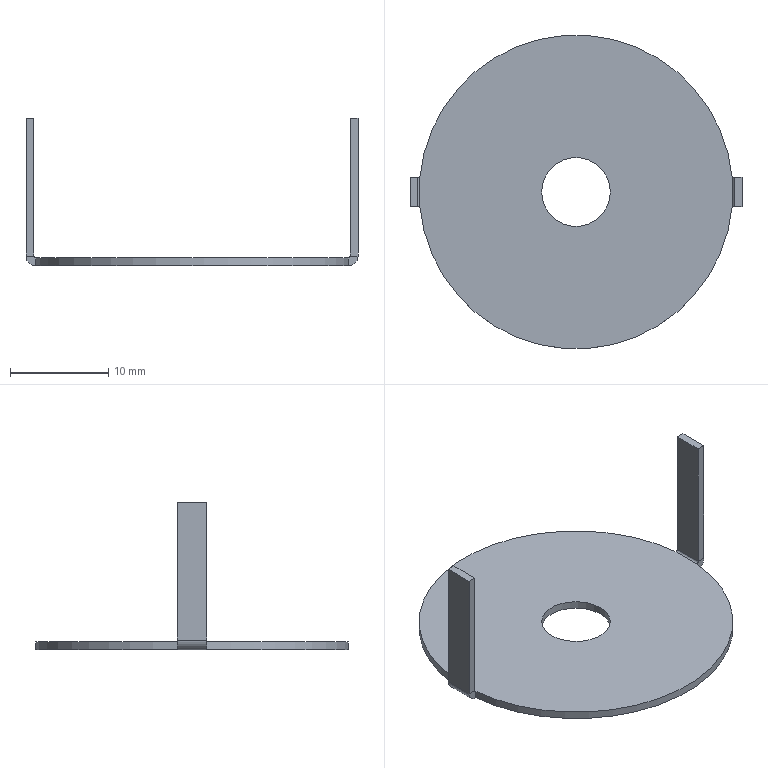Part | STEP file | Q7C1215W | 1 solid | 23 faces | box 33.859 x 32 x 15.058 mm | volume 684.385 mm3 | plane 16 | cylinder 7 | commonest cylinder face diameters 0.4 x2 2 x2 32 x2 7 x1
STEP:
#1=CARTESIAN_POINT('',(0.,0.,0.));
#2=DIRECTION('',(0.,0.,1.));
#3=DIRECTION('',(1.,0.,0.));
#4=AXIS2_PLACEMENT_3D('',#1,#2,#3);
#5=CARTESIAN_POINT('',(3.5,0.,0.));
#6=VERTEX_POINT('',#5);
#7=CARTESIAN_POINT('',(0.,0.,0.));
#8=DIRECTION('',(0.,0.,1.));
#9=DIRECTION('',(1.,0.,0.));
#10=AXIS2_PLACEMENT_3D('',#7,#8,#9);
#11=CIRCLE('',#10,3.5);
#12=CARTESIAN_POINT('',(0.,0.,0.));
#13=DIRECTION('',(0.,0.,1.));
#14=DIRECTION('',(1.,0.,0.));
#15=AXIS2_PLACEMENT_3D('',#12,#13,#14);
#16=PLANE('',#15);
#17=CARTESIAN_POINT('',(0.,0.));
#18=DIRECTION('',(1.,0.));
#19=AXIS2_PLACEMENT_2D('',#17,#18);
#20=CIRCLE('',#19,3.5);
#21=(GEOMETRIC_REPRESENTATION_CONTEXT(2)PARAMETRIC_REPRESENTATION_CONTEXT()REPRESENTATION_CONTEXT('',''));
#22=DEFINITIONAL_REPRESENTATION('',(#20),#21);
#23=PCURVE('',#16,#22);
#24=CARTESIAN_POINT('',(0.,0.,-0.8));
#25=DIRECTION('',(0.,0.,1.));
#26=DIRECTION('',(1.,0.,0.));
#27=AXIS2_PLACEMENT_3D('',#24,#25,#26);
#28=CYLINDRICAL_SURFACE('',#27,3.5);
#29=CARTESIAN_POINT('',(0.,0.8));
#30=DIRECTION('',(1.,0.));
#31=VECTOR('',#30,1.);
#32=LINE('',#29,#31);
#33=(GEOMETRIC_REPRESENTATION_CONTEXT(2)PARAMETRIC_REPRESENTATION_CONTEXT()REPRESENTATION_CONTEXT('',''));
#34=DEFINITIONAL_REPRESENTATION('',(#32),#33);
#35=PCURVE('',#28,#34);
#36=SURFACE_CURVE('',#11,(#23,#35),.PCURVE_S1.);
#37=EDGE_CURVE('',#6,#6,#36,.T.);
#38=ORIENTED_EDGE('',*,*,#37,.F.);
#39=EDGE_LOOP('',(#38));
#40=FACE_BOUND('',#39,.T.);
#41=CARTESIAN_POINT('',(-15.93,-1.5,0.));
#42=VERTEX_POINT('',#41);
#43=CARTESIAN_POINT('',(15.93,-1.5,0.));
#44=VERTEX_POINT('',#43);
#45=CARTESIAN_POINT('',(0.,0.,0.));
#46=DIRECTION('',(0.,0.,1.));
#47=DIRECTION('',(1.,0.,0.));
#48=AXIS2_PLACEMENT_3D('',#45,#46,#47);
#49=CIRCLE('',#48,16.);
#50=CARTESIAN_POINT('',(0.,0.));
#51=DIRECTION('',(1.,0.));
#52=AXIS2_PLACEMENT_2D('',#50,#51);
#53=CIRCLE('',#52,16.);
#54=(GEOMETRIC_REPRESENTATION_CONTEXT(2)PARAMETRIC_REPRESENTATION_CONTEXT()REPRESENTATION_CONTEXT('',''));
#55=DEFINITIONAL_REPRESENTATION('',(#53),#54);
#56=PCURVE('',#16,#55);
#57=CARTESIAN_POINT('',(0.,0.,-0.8));
#58=DIRECTION('',(0.,0.,1.));
#59=DIRECTION('',(1.,0.,0.));
#60=AXIS2_PLACEMENT_3D('',#57,#58,#59);
#61=CYLINDRICAL_SURFACE('',#60,16.);
#62=CARTESIAN_POINT('',(0.,0.8));
#63=DIRECTION('',(1.,0.));
#64=VECTOR('',#63,1.);
#65=LINE('',#62,#64);
#66=(GEOMETRIC_REPRESENTATION_CONTEXT(2)PARAMETRIC_REPRESENTATION_CONTEXT()REPRESENTATION_CONTEXT('',''));
#67=DEFINITIONAL_REPRESENTATION('',(#65),#66);
#68=PCURVE('',#61,#67);
#69=SURFACE_CURVE('',#49,(#56,#68),.PCURVE_S1.);
#70=EDGE_CURVE('',#42,#44,#69,.T.);
#71=ORIENTED_EDGE('',*,*,#70,.T.);
#72=CARTESIAN_POINT('',(15.93,1.5,0.));
#73=VERTEX_POINT('',#72);
#74=CARTESIAN_POINT('',(15.93,0.,0.));
#75=DIRECTION('',(0.,1.,0.));
#76=VECTOR('',#75,1.);
#77=LINE('',#74,#76);
#78=CARTESIAN_POINT('',(15.93,0.));
#79=DIRECTION('',(0.,1.));
#80=VECTOR('',#79,1.);
#81=LINE('',#78,#80);
#82=(GEOMETRIC_REPRESENTATION_CONTEXT(2)PARAMETRIC_REPRESENTATION_CONTEXT()REPRESENTATION_CONTEXT('',''));
#83=DEFINITIONAL_REPRESENTATION('',(#81),#82);
#84=PCURVE('',#16,#83);
#85=CARTESIAN_POINT('',(15.93,3.245,0.2));
#86=DIRECTION('',(0.,-1.,0.));
#87=DIRECTION('',(0.,0.,-1.));
#88=AXIS2_PLACEMENT_3D('',#85,#86,#87);
#89=CYLINDRICAL_SURFACE('',#88,0.2);
#90=CARTESIAN_POINT('',(0.,3.245));
#91=DIRECTION('',(0.,-1.));
#92=VECTOR('',#91,1.);
#93=LINE('',#90,#92);
#94=(GEOMETRIC_REPRESENTATION_CONTEXT(2)PARAMETRIC_REPRESENTATION_CONTEXT()REPRESENTATION_CONTEXT('',''));
#95=DEFINITIONAL_REPRESENTATION('',(#93),#94);
#96=PCURVE('',#89,#95);
#97=SURFACE_CURVE('',#77,(#84,#96),.PCURVE_S1.);
#98=EDGE_CURVE('',#44,#73,#97,.T.);
#99=ORIENTED_EDGE('',*,*,#98,.T.);
#100=CARTESIAN_POINT('',(-15.93,1.5,0.));
#101=VERTEX_POINT('',#100);
#102=CARTESIAN_POINT('',(0.,0.,0.));
#103=DIRECTION('',(0.,0.,1.));
#104=DIRECTION('',(1.,0.,0.));
#105=AXIS2_PLACEMENT_3D('',#102,#103,#104);
#106=CIRCLE('',#105,16.);
#107=CARTESIAN_POINT('',(0.,0.));
#108=DIRECTION('',(1.,0.));
#109=AXIS2_PLACEMENT_2D('',#107,#108);
#110=CIRCLE('',#109,16.);
#111=(GEOMETRIC_REPRESENTATION_CONTEXT(2)PARAMETRIC_REPRESENTATION_CONTEXT()REPRESENTATION_CONTEXT('',''));
#112=DEFINITIONAL_REPRESENTATION('',(#110),#111);
#113=PCURVE('',#16,#112);
#114=CARTESIAN_POINT('',(0.,0.,-0.8));
#115=DIRECTION('',(0.,0.,1.));
#116=DIRECTION('',(1.,0.,0.));
#117=AXIS2_PLACEMENT_3D('',#114,#115,#116);
#118=CYLINDRICAL_SURFACE('',#117,16.);
#119=CARTESIAN_POINT('',(0.,0.8));
#120=DIRECTION('',(1.,0.));
#121=VECTOR('',#120,1.);
#122=LINE('',#119,#121);
#123=(GEOMETRIC_REPRESENTATION_CONTEXT(2)PARAMETRIC_REPRESENTATION_CONTEXT()REPRESENTATION_CONTEXT('',''));
#124=DEFINITIONAL_REPRESENTATION('',(#122),#123);
#125=PCURVE('',#118,#124);
#126=SURFACE_CURVE('',#106,(#113,#125),.PCURVE_S1.);
#127=EDGE_CURVE('',#73,#101,#126,.T.);
#128=ORIENTED_EDGE('',*,*,#127,.T.);
#129=CARTESIAN_POINT('',(-15.93,0.,0.));
#130=DIRECTION('',(0.,1.,0.));
#131=VECTOR('',#130,1.);
#132=LINE('',#129,#131);
#133=CARTESIAN_POINT('',(-15.93,0.));
#134=DIRECTION('',(0.,1.));
#135=VECTOR('',#134,1.);
#136=LINE('',#133,#135);
#137=(GEOMETRIC_REPRESENTATION_CONTEXT(2)PARAMETRIC_REPRESENTATION_CONTEXT()REPRESENTATION_CONTEXT('',''));
#138=DEFINITIONAL_REPRESENTATION('',(#136),#137);
#139=PCURVE('',#16,#138);
#140=CARTESIAN_POINT('',(-15.93,-3.245,0.2));
#141=DIRECTION('',(0.,1.,0.));
#142=DIRECTION('',(0.,0.,1.));
#143=AXIS2_PLACEMENT_3D('',#140,#141,#142);
#144=CYLINDRICAL_SURFACE('',#143,0.2);
#145=CARTESIAN_POINT('',(3.142,3.245));
#146=DIRECTION('',(0.,1.));
#147=VECTOR('',#146,1.);
#148=LINE('',#145,#147);
#149=(GEOMETRIC_REPRESENTATION_CONTEXT(2)PARAMETRIC_REPRESENTATION_CONTEXT()REPRESENTATION_CONTEXT('',''));
#150=DEFINITIONAL_REPRESENTATION('',(#148),#149);
#151=PCURVE('',#144,#150);
#152=SURFACE_CURVE('',#132,(#139,#151),.PCURVE_S1.);
#153=EDGE_CURVE('',#42,#101,#152,.T.);
#154=ORIENTED_EDGE('',*,*,#153,.F.);
#155=EDGE_LOOP('',(#71,#99,#128,#154));
#156=FACE_BOUND('',#155,.T.);
#157=ADVANCED_FACE('',(#40,#156),#16,.T.);
#158=CARTESIAN_POINT('',(15.93,-1.5,-0.8));
#159=VERTEX_POINT('',#158);
#160=CARTESIAN_POINT('',(15.93,1.5,-0.8));
#161=VERTEX_POINT('',#160);
#162=CARTESIAN_POINT('',(15.93,0.,-0.8));
#163=DIRECTION('',(0.,1.,0.));
#164=VECTOR('',#163,1.);
#165=LINE('',#162,#164);
#166=CARTESIAN_POINT('',(0.,0.,-0.8));
#167=DIRECTION('',(0.,0.,1.));
#168=DIRECTION('',(1.,0.,0.));
#169=AXIS2_PLACEMENT_3D('',#166,#167,#168);
#170=PLANE('',#169);
#171=CARTESIAN_POINT('',(15.93,0.));
#172=DIRECTION('',(0.,1.));
#173=VECTOR('',#172,1.);
#174=LINE('',#171,#173);
#175=(GEOMETRIC_REPRESENTATION_CONTEXT(2)PARAMETRIC_REPRESENTATION_CONTEXT()REPRESENTATION_CONTEXT('',''));
#176=DEFINITIONAL_REPRESENTATION('',(#174),#175);
#177=PCURVE('',#170,#176);
#178=CARTESIAN_POINT('',(15.93,3.245,0.2));
#179=DIRECTION('',(0.,-1.,0.));
#180=DIRECTION('',(0.,0.,-1.));
#181=AXIS2_PLACEMENT_3D('',#178,#179,#180);
#182=CYLINDRICAL_SURFACE('',#181,1.);
#183=CARTESIAN_POINT('',(0.,3.245));
#184=DIRECTION('',(0.,-1.));
#185=VECTOR('',#184,1.);
#186=LINE('',#183,#185);
#187=(GEOMETRIC_REPRESENTATION_CONTEXT(2)PARAMETRIC_REPRESENTATION_CONTEXT()REPRESENTATION_CONTEXT('',''));
#188=DEFINITIONAL_REPRESENTATION('',(#186),#187);
#189=PCURVE('',#182,#188);
#190=SURFACE_CURVE('',#165,(#177,#189),.PCURVE_S1.);
#191=EDGE_CURVE('',#159,#161,#190,.T.);
#192=ORIENTED_EDGE('',*,*,#191,.F.);
#193=CARTESIAN_POINT('',(-15.93,-1.5,-0.8));
#194=VERTEX_POINT('',#193);
#195=CARTESIAN_POINT('',(0.,0.,-0.8));
#196=DIRECTION('',(0.,0.,1.));
#197=DIRECTION('',(1.,0.,0.));
#198=AXIS2_PLACEMENT_3D('',#195,#196,#197);
#199=CIRCLE('',#198,16.);
#200=CARTESIAN_POINT('',(0.,0.));
#201=DIRECTION('',(1.,0.));
#202=AXIS2_PLACEMENT_2D('',#200,#201);
#203=CIRCLE('',#202,16.);
#204=(GEOMETRIC_REPRESENTATION_CONTEXT(2)PARAMETRIC_REPRESENTATION_CONTEXT()REPRESENTATION_CONTEXT('',''));
#205=DEFINITIONAL_REPRESENTATION('',(#203),#204);
#206=PCURVE('',#170,#205);
#207=CARTESIAN_POINT('',(0.,0.));
#208=DIRECTION('',(1.,0.));
#209=VECTOR('',#208,1.);
#210=LINE('',#207,#209);
#211=(GEOMETRIC_REPRESENTATION_CONTEXT(2)PARAMETRIC_REPRESENTATION_CONTEXT()REPRESENTATION_CONTEXT('',''));
#212=DEFINITIONAL_REPRESENTATION('',(#210),#211);
#213=PCURVE('',#61,#212);
#214=SURFACE_CURVE('',#199,(#206,#213),.PCURVE_S1.);
#215=EDGE_CURVE('',#194,#159,#214,.T.);
#216=ORIENTED_EDGE('',*,*,#215,.F.);
#217=CARTESIAN_POINT('',(-15.93,1.5,-0.8));
#218=VERTEX_POINT('',#217);
#219=CARTESIAN_POINT('',(-15.93,0.,-0.8));
#220=DIRECTION('',(0.,1.,0.));
#221=VECTOR('',#220,1.);
#222=LINE('',#219,#221);
#223=CARTESIAN_POINT('',(-15.93,0.));
#224=DIRECTION('',(0.,1.));
#225=VECTOR('',#224,1.);
#226=LINE('',#223,#225);
#227=(GEOMETRIC_REPRESENTATION_CONTEXT(2)PARAMETRIC_REPRESENTATION_CONTEXT()REPRESENTATION_CONTEXT('',''));
#228=DEFINITIONAL_REPRESENTATION('',(#226),#227);
#229=PCURVE('',#170,#228);
#230=CARTESIAN_POINT('',(-15.93,-3.245,0.2));
#231=DIRECTION('',(0.,1.,0.));
#232=DIRECTION('',(0.,0.,1.));
#233=AXIS2_PLACEMENT_3D('',#230,#231,#232);
#234=CYLINDRICAL_SURFACE('',#233,1.);
#235=CARTESIAN_POINT('',(3.142,3.245));
#236=DIRECTION('',(0.,1.));
#237=VECTOR('',#236,1.);
#238=LINE('',#235,#237);
#239=(GEOMETRIC_REPRESENTATION_CONTEXT(2)PARAMETRIC_REPRESENTATION_CONTEXT()REPRESENTATION_CONTEXT('',''));
#240=DEFINITIONAL_REPRESENTATION('',(#238),#239);
#241=PCURVE('',#234,#240);
#242=SURFACE_CURVE('',#222,(#229,#241),.PCURVE_S1.);
#243=EDGE_CURVE('',#194,#218,#242,.T.);
#244=ORIENTED_EDGE('',*,*,#243,.T.);
#245=CARTESIAN_POINT('',(0.,0.,-0.8));
#246=DIRECTION('',(0.,0.,1.));
#247=DIRECTION('',(1.,0.,0.));
#248=AXIS2_PLACEMENT_3D('',#245,#246,#247);
#249=CIRCLE('',#248,16.);
#250=CARTESIAN_POINT('',(0.,0.));
#251=DIRECTION('',(1.,0.));
#252=AXIS2_PLACEMENT_2D('',#250,#251);
#253=CIRCLE('',#252,16.);
#254=(GEOMETRIC_REPRESENTATION_CONTEXT(2)PARAMETRIC_REPRESENTATION_CONTEXT()REPRESENTATION_CONTEXT('',''));
#255=DEFINITIONAL_REPRESENTATION('',(#253),#254);
#256=PCURVE('',#170,#255);
#257=CARTESIAN_POINT('',(0.,0.));
#258=DIRECTION('',(1.,0.));
#259=VECTOR('',#258,1.);
#260=LINE('',#257,#259);
#261=(GEOMETRIC_REPRESENTATION_CONTEXT(2)PARAMETRIC_REPRESENTATION_CONTEXT()REPRESENTATION_CONTEXT('',''));
#262=DEFINITIONAL_REPRESENTATION('',(#260),#261);
#263=PCURVE('',#118,#262);
#264=SURFACE_CURVE('',#249,(#256,#263),.PCURVE_S1.);
#265=EDGE_CURVE('',#161,#218,#264,.T.);
#266=ORIENTED_EDGE('',*,*,#265,.F.);
#267=EDGE_LOOP('',(#192,#216,#244,#266));
#268=FACE_BOUND('',#267,.T.);
#269=CARTESIAN_POINT('',(3.5,0.,-0.8));
#270=VERTEX_POINT('',#269);
#271=CARTESIAN_POINT('',(0.,0.,-0.8));
#272=DIRECTION('',(0.,0.,1.));
#273=DIRECTION('',(1.,0.,0.));
#274=AXIS2_PLACEMENT_3D('',#271,#272,#273);
#275=CIRCLE('',#274,3.5);
#276=CARTESIAN_POINT('',(0.,0.));
#277=DIRECTION('',(1.,0.));
#278=AXIS2_PLACEMENT_2D('',#276,#277);
#279=CIRCLE('',#278,3.5);
#280=(GEOMETRIC_REPRESENTATION_CONTEXT(2)PARAMETRIC_REPRESENTATION_CONTEXT()REPRESENTATION_CONTEXT('',''));
#281=DEFINITIONAL_REPRESENTATION('',(#279),#280);
#282=PCURVE('',#170,#281);
#283=CARTESIAN_POINT('',(0.,0.));
#284=DIRECTION('',(1.,0.));
#285=VECTOR('',#284,1.);
#286=LINE('',#283,#285);
#287=(GEOMETRIC_REPRESENTATION_CONTEXT(2)PARAMETRIC_REPRESENTATION_CONTEXT()REPRESENTATION_CONTEXT('',''));
#288=DEFINITIONAL_REPRESENTATION('',(#286),#287);
#289=PCURVE('',#28,#288);
#290=SURFACE_CURVE('',#275,(#282,#289),.PCURVE_S1.);
#291=EDGE_CURVE('',#270,#270,#290,.T.);
#292=ORIENTED_EDGE('',*,*,#291,.T.);
#293=EDGE_LOOP('',(#292));
#294=FACE_BOUND('',#293,.T.);
#295=ADVANCED_FACE('',(#268,#294),#170,.F.);
#296=ORIENTED_EDGE('',*,*,#127,.F.);
#297=CARTESIAN_POINT('',(15.93,1.5,-0.8));
#298=DIRECTION('',(0.,0.,1.));
#299=VECTOR('',#298,1.);
#300=LINE('',#297,#299);
#301=CARTESIAN_POINT('',(0.09389,0.));
#302=DIRECTION('',(0.,1.));
#303=VECTOR('',#302,1.);
#304=LINE('',#301,#303);
#305=(GEOMETRIC_REPRESENTATION_CONTEXT(2)PARAMETRIC_REPRESENTATION_CONTEXT()REPRESENTATION_CONTEXT('',''));
#306=DEFINITIONAL_REPRESENTATION('',(#304),#305);
#307=PCURVE('',#118,#306);
#308=CARTESIAN_POINT('',(15.93,1.5,0.2));
#309=DIRECTION('',(0.,1.,0.));
#310=DIRECTION('',(0.,0.,1.));
#311=AXIS2_PLACEMENT_3D('',#308,#309,#310);
#312=PLANE('',#311);
#313=CARTESIAN_POINT('',(-1.,0.));
#314=DIRECTION('',(1.,0.));
#315=VECTOR('',#314,1.);
#316=LINE('',#313,#315);
#317=(GEOMETRIC_REPRESENTATION_CONTEXT(2)PARAMETRIC_REPRESENTATION_CONTEXT()REPRESENTATION_CONTEXT('',''));
#318=DEFINITIONAL_REPRESENTATION('',(#316),#317);
#319=PCURVE('',#312,#318);
#320=SURFACE_CURVE('',#300,(#307,#319),.PCURVE_S1.);
#321=EDGE_CURVE('',#161,#73,#320,.T.);
#322=ORIENTED_EDGE('',*,*,#321,.F.);
#323=ORIENTED_EDGE('',*,*,#265,.T.);
#324=CARTESIAN_POINT('',(-15.93,1.5,-0.8));
#325=DIRECTION('',(0.,0.,1.));
#326=VECTOR('',#325,1.);
#327=LINE('',#324,#326);
#328=CARTESIAN_POINT('',(3.048,0.));
#329=DIRECTION('',(0.,1.));
#330=VECTOR('',#329,1.);
#331=LINE('',#328,#330);
#332=(GEOMETRIC_REPRESENTATION_CONTEXT(2)PARAMETRIC_REPRESENTATION_CONTEXT()REPRESENTATION_CONTEXT('',''));
#333=DEFINITIONAL_REPRESENTATION('',(#331),#332);
#334=PCURVE('',#118,#333);
#335=CARTESIAN_POINT('',(-15.93,1.5,0.2));
#336=DIRECTION('',(0.,1.,0.));
#337=DIRECTION('',(0.,0.,1.));
#338=AXIS2_PLACEMENT_3D('',#335,#336,#337);
#339=PLANE('',#338);
#340=CARTESIAN_POINT('',(-1.,0.));
#341=DIRECTION('',(1.,0.));
#342=VECTOR('',#341,1.);
#343=LINE('',#340,#342);
#344=(GEOMETRIC_REPRESENTATION_CONTEXT(2)PARAMETRIC_REPRESENTATION_CONTEXT()REPRESENTATION_CONTEXT('',''));
#345=DEFINITIONAL_REPRESENTATION('',(#343),#344);
#346=PCURVE('',#339,#345);
#347=SURFACE_CURVE('',#327,(#334,#346),.PCURVE_S1.);
#348=EDGE_CURVE('',#218,#101,#347,.T.);
#349=ORIENTED_EDGE('',*,*,#348,.T.);
#350=EDGE_LOOP('',(#296,#322,#323,#349));
#351=FACE_BOUND('',#350,.T.);
#352=ADVANCED_FACE('',(#351),#118,.T.);
#353=ORIENTED_EDGE('',*,*,#70,.F.);
#354=CARTESIAN_POINT('',(-15.93,-1.5,-0.8));
#355=DIRECTION('',(0.,0.,1.));
#356=VECTOR('',#355,1.);
#357=LINE('',#354,#356);
#358=CARTESIAN_POINT('',(3.235,0.));
#359=DIRECTION('',(0.,1.));
#360=VECTOR('',#359,1.);
#361=LINE('',#358,#360);
#362=(GEOMETRIC_REPRESENTATION_CONTEXT(2)PARAMETRIC_REPRESENTATION_CONTEXT()REPRESENTATION_CONTEXT('',''));
#363=DEFINITIONAL_REPRESENTATION('',(#361),#362);
#364=PCURVE('',#61,#363);
#365=CARTESIAN_POINT('',(-15.93,-1.5,0.2));
#366=DIRECTION('',(0.,-1.,0.));
#367=DIRECTION('',(0.,0.,-1.));
#368=AXIS2_PLACEMENT_3D('',#365,#366,#367);
#369=PLANE('',#368);
#370=CARTESIAN_POINT('',(1.,0.));
#371=DIRECTION('',(-1.,0.));
#372=VECTOR('',#371,1.);
#373=LINE('',#370,#372);
#374=(GEOMETRIC_REPRESENTATION_CONTEXT(2)PARAMETRIC_REPRESENTATION_CONTEXT()REPRESENTATION_CONTEXT('',''));
#375=DEFINITIONAL_REPRESENTATION('',(#373),#374);
#376=PCURVE('',#369,#375);
#377=SURFACE_CURVE('',#357,(#364,#376),.PCURVE_S1.);
#378=EDGE_CURVE('',#194,#42,#377,.T.);
#379=ORIENTED_EDGE('',*,*,#378,.F.);
#380=ORIENTED_EDGE('',*,*,#215,.T.);
#381=CARTESIAN_POINT('',(15.93,-1.5,-0.8));
#382=DIRECTION('',(0.,0.,1.));
#383=VECTOR('',#382,1.);
#384=LINE('',#381,#383);
#385=CARTESIAN_POINT('',(6.189,0.));
#386=DIRECTION('',(0.,1.));
#387=VECTOR('',#386,1.);
#388=LINE('',#385,#387);
#389=(GEOMETRIC_REPRESENTATION_CONTEXT(2)PARAMETRIC_REPRESENTATION_CONTEXT()REPRESENTATION_CONTEXT('',''));
#390=DEFINITIONAL_REPRESENTATION('',(#388),#389);
#391=PCURVE('',#61,#390);
#392=CARTESIAN_POINT('',(15.93,-1.5,0.2));
#393=DIRECTION('',(0.,-1.,0.));
#394=DIRECTION('',(1.,0.,0.));
#395=AXIS2_PLACEMENT_3D('',#392,#393,#394);
#396=PLANE('',#395);
#397=CARTESIAN_POINT('',(0.,-1.));
#398=DIRECTION('',(0.,1.));
#399=VECTOR('',#398,1.);
#400=LINE('',#397,#399);
#401=(GEOMETRIC_REPRESENTATION_CONTEXT(2)PARAMETRIC_REPRESENTATION_CONTEXT()REPRESENTATION_CONTEXT('',''));
#402=DEFINITIONAL_REPRESENTATION('',(#400),#401);
#403=PCURVE('',#396,#402);
#404=SURFACE_CURVE('',#384,(#391,#403),.PCURVE_S1.);
#405=EDGE_CURVE('',#159,#44,#404,.T.);
#406=ORIENTED_EDGE('',*,*,#405,.T.);
#407=EDGE_LOOP('',(#353,#379,#380,#406));
#408=FACE_BOUND('',#407,.T.);
#409=ADVANCED_FACE('',(#408),#61,.T.);
#410=ORIENTED_EDGE('',*,*,#291,.T.);
#411=CARTESIAN_POINT('',(3.5,0.,-0.8));
#412=CARTESIAN_POINT('',(3.5,0.,0.));
#413=B_SPLINE_CURVE_WITH_KNOTS('',1,(#411,#412),.UNSPECIFIED.,.F.,.F.,(2,2),(0.,0.8),.PIECEWISE_BEZIER_KNOTS.);
#414=CARTESIAN_POINT('',(6.283,0.));
#415=DIRECTION('',(0.,1.));
#416=VECTOR('',#415,1.);
#417=LINE('',#414,#416);
#418=(GEOMETRIC_REPRESENTATION_CONTEXT(2)PARAMETRIC_REPRESENTATION_CONTEXT()REPRESENTATION_CONTEXT('',''));
#419=DEFINITIONAL_REPRESENTATION('',(#417),#418);
#420=PCURVE('',#28,#419);
#421=CARTESIAN_POINT('',(0.,0.));
#422=DIRECTION('',(0.,1.));
#423=VECTOR('',#422,1.);
#424=LINE('',#421,#423);
#425=(GEOMETRIC_REPRESENTATION_CONTEXT(2)PARAMETRIC_REPRESENTATION_CONTEXT()REPRESENTATION_CONTEXT('',''));
#426=DEFINITIONAL_REPRESENTATION('',(#424),#425);
#427=PCURVE('',#28,#426);
#428=SEAM_CURVE('',#413,(#420,#427),.PCURVE_S1.);
#429=EDGE_CURVE('',#270,#6,#428,.T.);
#430=ORIENTED_EDGE('',*,*,#429,.T.);
#431=ORIENTED_EDGE('',*,*,#37,.F.);
#432=ORIENTED_EDGE('',*,*,#429,.F.);
#433=EDGE_LOOP('',(#410,#430,#431,#432));
#434=FACE_BOUND('',#433,.F.);
#435=ADVANCED_FACE('',(#434),#28,.F.);
#436=ORIENTED_EDGE('',*,*,#378,.T.);
#437=CARTESIAN_POINT('',(-16.13,-1.5,0.2));
#438=VERTEX_POINT('',#437);
#439=CARTESIAN_POINT('',(-15.93,-1.5,0.2));
#440=DIRECTION('',(0.,1.,0.));
#441=DIRECTION('',(0.,0.,1.));
#442=AXIS2_PLACEMENT_3D('',#439,#440,#441);
#443=CIRCLE('',#442,0.2);
#444=CARTESIAN_POINT('',(-0.2,0.));
#445=CARTESIAN_POINT('',(-0.2,0.3464));
#446=CARTESIAN_POINT('',(0.1,0.1732));
#447=CARTESIAN_POINT('',(0.4,0.));
#448=CARTESIAN_POINT('',(0.1,-0.1732));
#449=CARTESIAN_POINT('',(-0.2,-0.3464));
#450=CARTESIAN_POINT('',(-0.2,0.));
#451=(BOUNDED_CURVE()B_SPLINE_CURVE(2,(#444,#445,#446,#447,#448,#449,#450),.UNSPECIFIED.,.T.,.F.)B_SPLINE_CURVE_WITH_KNOTS((1,2,2,2,2,1),(-2.094,0.,2.094,4.189,6.283,8.378),.UNSPECIFIED.)CURVE()GEOMETRIC_REPRESENTATION_ITEM()RATIONAL_B_SPLINE_CURVE((1.,0.5,1.,0.5,1.,0.5,1.))REPRESENTATION_ITEM(''));
#452=(GEOMETRIC_REPRESENTATION_CONTEXT(2)PARAMETRIC_REPRESENTATION_CONTEXT()REPRESENTATION_CONTEXT('',''));
#453=DEFINITIONAL_REPRESENTATION('',(#451),#452);
#454=PCURVE('',#369,#453);
#455=CARTESIAN_POINT('',(0.,1.745));
#456=DIRECTION('',(1.,0.));
#457=VECTOR('',#456,1.);
#458=LINE('',#455,#457);
#459=(GEOMETRIC_REPRESENTATION_CONTEXT(2)PARAMETRIC_REPRESENTATION_CONTEXT()REPRESENTATION_CONTEXT('',''));
#460=DEFINITIONAL_REPRESENTATION('',(#458),#459);
#461=PCURVE('',#144,#460);
#462=SURFACE_CURVE('',#443,(#454,#461),.PCURVE_S1.);
#463=EDGE_CURVE('',#42,#438,#462,.T.);
#464=ORIENTED_EDGE('',*,*,#463,.T.);
#465=CARTESIAN_POINT('',(-16.93,-1.5,0.2));
#466=VERTEX_POINT('',#465);
#467=CARTESIAN_POINT('',(-16.93,-1.5,0.2));
#468=DIRECTION('',(1.,0.,0.));
#469=VECTOR('',#468,1.);
#470=LINE('',#467,#469);
#471=CARTESIAN_POINT('',(0.,-1.));
#472=DIRECTION('',(0.,1.));
#473=VECTOR('',#472,1.);
#474=LINE('',#471,#473);
#475=(GEOMETRIC_REPRESENTATION_CONTEXT(2)PARAMETRIC_REPRESENTATION_CONTEXT()REPRESENTATION_CONTEXT('',''));
#476=DEFINITIONAL_REPRESENTATION('',(#474),#475);
#477=PCURVE('',#369,#476);
#478=CARTESIAN_POINT('',(-16.93,-1.5,-0.7425));
#479=DIRECTION('',(0.,-1.,0.));
#480=DIRECTION('',(-1.,0.,0.));
#481=AXIS2_PLACEMENT_3D('',#478,#479,#480);
#482=PLANE('',#481);
#483=CARTESIAN_POINT('',(0.,-0.9425));
#484=DIRECTION('',(-1.,0.));
#485=VECTOR('',#484,1.);
#486=LINE('',#483,#485);
#487=(GEOMETRIC_REPRESENTATION_CONTEXT(2)PARAMETRIC_REPRESENTATION_CONTEXT()REPRESENTATION_CONTEXT('',''));
#488=DEFINITIONAL_REPRESENTATION('',(#486),#487);
#489=PCURVE('',#482,#488);
#490=SURFACE_CURVE('',#470,(#477,#489),.PCURVE_S1.);
#491=EDGE_CURVE('',#466,#438,#490,.T.);
#492=ORIENTED_EDGE('',*,*,#491,.F.);
#493=CARTESIAN_POINT('',(-15.93,-1.5,0.2));
#494=DIRECTION('',(0.,1.,0.));
#495=DIRECTION('',(0.,0.,-1.));
#496=AXIS2_PLACEMENT_3D('',#493,#494,#495);
#497=CIRCLE('',#496,1.);
#498=CARTESIAN_POINT('',(1.,0.));
#499=CARTESIAN_POINT('',(1.,-1.732));
#500=CARTESIAN_POINT('',(-0.5,-0.866));
#501=CARTESIAN_POINT('',(-2.,0.));
#502=CARTESIAN_POINT('',(-0.5,0.866));
#503=CARTESIAN_POINT('',(1.,1.732));
#504=CARTESIAN_POINT('',(1.,0.));
#505=(BOUNDED_CURVE()B_SPLINE_CURVE(2,(#498,#499,#500,#501,#502,#503,#504),.UNSPECIFIED.,.T.,.F.)B_SPLINE_CURVE_WITH_KNOTS((1,2,2,2,2,1),(-2.094,0.,2.094,4.189,6.283,8.378),.UNSPECIFIED.)CURVE()GEOMETRIC_REPRESENTATION_ITEM()RATIONAL_B_SPLINE_CURVE((1.,0.5,1.,0.5,1.,0.5,1.))REPRESENTATION_ITEM(''));
#506=(GEOMETRIC_REPRESENTATION_CONTEXT(2)PARAMETRIC_REPRESENTATION_CONTEXT()REPRESENTATION_CONTEXT('',''));
#507=DEFINITIONAL_REPRESENTATION('',(#505),#506);
#508=PCURVE('',#369,#507);
#509=CARTESIAN_POINT('',(3.142,1.745));
#510=DIRECTION('',(1.,0.));
#511=VECTOR('',#510,1.);
#512=LINE('',#509,#511);
#513=(GEOMETRIC_REPRESENTATION_CONTEXT(2)PARAMETRIC_REPRESENTATION_CONTEXT()REPRESENTATION_CONTEXT('',''));
#514=DEFINITIONAL_REPRESENTATION('',(#512),#513);
#515=PCURVE('',#234,#514);
#516=SURFACE_CURVE('',#497,(#508,#515),.PCURVE_S1.);
#517=EDGE_CURVE('',#194,#466,#516,.T.);
#518=ORIENTED_EDGE('',*,*,#517,.F.);
#519=EDGE_LOOP('',(#436,#464,#492,#518));
#520=FACE_BOUND('',#519,.T.);
#521=ADVANCED_FACE('',(#520),#369,.T.);
#522=CARTESIAN_POINT('',(-16.13,1.5,0.2));
#523=VERTEX_POINT('',#522);
#524=CARTESIAN_POINT('',(-16.93,1.5,0.2));
#525=VERTEX_POINT('',#524);
#526=CARTESIAN_POINT('',(-16.93,1.5,0.2));
#527=DIRECTION('',(-1.,0.,0.));
#528=VECTOR('',#527,1.);
#529=LINE('',#526,#528);
#530=CARTESIAN_POINT('',(0.,-1.));
#531=DIRECTION('',(0.,-1.));
#532=VECTOR('',#531,1.);
#533=LINE('',#530,#532);
#534=(GEOMETRIC_REPRESENTATION_CONTEXT(2)PARAMETRIC_REPRESENTATION_CONTEXT()REPRESENTATION_CONTEXT('',''));
#535=DEFINITIONAL_REPRESENTATION('',(#533),#534);
#536=PCURVE('',#339,#535);
#537=CARTESIAN_POINT('',(-16.93,1.5,-0.7425));
#538=DIRECTION('',(0.,1.,0.));
#539=DIRECTION('',(1.,0.,0.));
#540=AXIS2_PLACEMENT_3D('',#537,#538,#539);
#541=PLANE('',#540);
#542=CARTESIAN_POINT('',(0.,-0.9425));
#543=DIRECTION('',(-1.,0.));
#544=VECTOR('',#543,1.);
#545=LINE('',#542,#544);
#546=(GEOMETRIC_REPRESENTATION_CONTEXT(2)PARAMETRIC_REPRESENTATION_CONTEXT()REPRESENTATION_CONTEXT('',''));
#547=DEFINITIONAL_REPRESENTATION('',(#545),#546);
#548=PCURVE('',#541,#547);
#549=SURFACE_CURVE('',#529,(#536,#548),.PCURVE_S1.);
#550=EDGE_CURVE('',#523,#525,#549,.T.);
#551=ORIENTED_EDGE('',*,*,#550,.F.);
#552=CARTESIAN_POINT('',(-15.93,1.5,0.2));
#553=DIRECTION('',(0.,-1.,0.));
#554=DIRECTION('',(0.,0.,1.));
#555=AXIS2_PLACEMENT_3D('',#552,#553,#554);
#556=CIRCLE('',#555,0.2);
#557=CARTESIAN_POINT('',(0.2,0.));
#558=CARTESIAN_POINT('',(0.2,-0.3464));
#559=CARTESIAN_POINT('',(-0.1,-0.1732));
#560=CARTESIAN_POINT('',(-0.4,0.));
#561=CARTESIAN_POINT('',(-0.1,0.1732));
#562=CARTESIAN_POINT('',(0.2,0.3464));
#563=CARTESIAN_POINT('',(0.2,0.));
#564=(BOUNDED_CURVE()B_SPLINE_CURVE(2,(#557,#558,#559,#560,#561,#562,#563),.UNSPECIFIED.,.T.,.F.)B_SPLINE_CURVE_WITH_KNOTS((1,2,2,2,2,1),(-2.094,0.,2.094,4.189,6.283,8.378),.UNSPECIFIED.)CURVE()GEOMETRIC_REPRESENTATION_ITEM()RATIONAL_B_SPLINE_CURVE((1.,0.5,1.,0.5,1.,0.5,1.))REPRESENTATION_ITEM(''));
#565=(GEOMETRIC_REPRESENTATION_CONTEXT(2)PARAMETRIC_REPRESENTATION_CONTEXT()REPRESENTATION_CONTEXT('',''));
#566=DEFINITIONAL_REPRESENTATION('',(#564),#565);
#567=PCURVE('',#339,#566);
#568=CARTESIAN_POINT('',(6.283,4.745));
#569=DIRECTION('',(-1.,0.));
#570=VECTOR('',#569,1.);
#571=LINE('',#568,#570);
#572=(GEOMETRIC_REPRESENTATION_CONTEXT(2)PARAMETRIC_REPRESENTATION_CONTEXT()REPRESENTATION_CONTEXT('',''));
#573=DEFINITIONAL_REPRESENTATION('',(#571),#572);
#574=PCURVE('',#144,#573);
#575=SURFACE_CURVE('',#556,(#567,#574),.PCURVE_S1.);
#576=EDGE_CURVE('',#523,#101,#575,.T.);
#577=ORIENTED_EDGE('',*,*,#576,.T.);
#578=ORIENTED_EDGE('',*,*,#348,.F.);
#579=CARTESIAN_POINT('',(-15.93,1.5,0.2));
#580=DIRECTION('',(0.,-1.,0.));
#581=DIRECTION('',(0.,0.,1.));
#582=AXIS2_PLACEMENT_3D('',#579,#580,#581);
#583=CIRCLE('',#582,1.);
#584=CARTESIAN_POINT('',(1.,0.));
#585=CARTESIAN_POINT('',(1.,-1.732));
#586=CARTESIAN_POINT('',(-0.5,-0.866));
#587=CARTESIAN_POINT('',(-2.,0.));
#588=CARTESIAN_POINT('',(-0.5,0.866));
#589=CARTESIAN_POINT('',(1.,1.732));
#590=CARTESIAN_POINT('',(1.,0.));
#591=(BOUNDED_CURVE()B_SPLINE_CURVE(2,(#584,#585,#586,#587,#588,#589,#590),.UNSPECIFIED.,.T.,.F.)B_SPLINE_CURVE_WITH_KNOTS((1,2,2,2,2,1),(-2.094,0.,2.094,4.189,6.283,8.378),.UNSPECIFIED.)CURVE()GEOMETRIC_REPRESENTATION_ITEM()RATIONAL_B_SPLINE_CURVE((1.,0.5,1.,0.5,1.,0.5,1.))REPRESENTATION_ITEM(''));
#592=(GEOMETRIC_REPRESENTATION_CONTEXT(2)PARAMETRIC_REPRESENTATION_CONTEXT()REPRESENTATION_CONTEXT('',''));
#593=DEFINITIONAL_REPRESENTATION('',(#591),#592);
#594=PCURVE('',#339,#593);
#595=CARTESIAN_POINT('',(6.283,4.745));
#596=DIRECTION('',(-1.,0.));
#597=VECTOR('',#596,1.);
#598=LINE('',#595,#597);
#599=(GEOMETRIC_REPRESENTATION_CONTEXT(2)PARAMETRIC_REPRESENTATION_CONTEXT()REPRESENTATION_CONTEXT('',''));
#600=DEFINITIONAL_REPRESENTATION('',(#598),#599);
#601=PCURVE('',#234,#600);
#602=SURFACE_CURVE('',#583,(#594,#601),.PCURVE_S1.);
#603=EDGE_CURVE('',#525,#218,#602,.T.);
#604=ORIENTED_EDGE('',*,*,#603,.F.);
#605=EDGE_LOOP('',(#551,#577,#578,#604));
#606=FACE_BOUND('',#605,.T.);
#607=ADVANCED_FACE('',(#606),#339,.T.);
#608=ORIENTED_EDGE('',*,*,#603,.T.);
#609=ORIENTED_EDGE('',*,*,#243,.F.);
#610=ORIENTED_EDGE('',*,*,#517,.T.);
#611=CARTESIAN_POINT('',(-16.93,0.,0.2));
#612=DIRECTION('',(0.,1.,0.));
#613=VECTOR('',#612,1.);
#614=LINE('',#611,#613);
#615=CARTESIAN_POINT('',(4.712,3.245));
#616=DIRECTION('',(0.,1.));
#617=VECTOR('',#616,1.);
#618=LINE('',#615,#617);
#619=(GEOMETRIC_REPRESENTATION_CONTEXT(2)PARAMETRIC_REPRESENTATION_CONTEXT()REPRESENTATION_CONTEXT('',''));
#620=DEFINITIONAL_REPRESENTATION('',(#618),#619);
#621=PCURVE('',#234,#620);
#622=CARTESIAN_POINT('',(-16.93,0.,-16.672));
#623=DIRECTION('',(1.,0.,0.));
#624=DIRECTION('',(0.,0.,-1.));
#625=AXIS2_PLACEMENT_3D('',#622,#623,#624);
#626=PLANE('',#625);
#627=CARTESIAN_POINT('',(-16.872,0.));
#628=DIRECTION('',(0.,1.));
#629=VECTOR('',#628,1.);
#630=LINE('',#627,#629);
#631=(GEOMETRIC_REPRESENTATION_CONTEXT(2)PARAMETRIC_REPRESENTATION_CONTEXT()REPRESENTATION_CONTEXT('',''));
#632=DEFINITIONAL_REPRESENTATION('',(#630),#631);
#633=PCURVE('',#626,#632);
#634=SURFACE_CURVE('',#614,(#621,#633),.PCURVE_S1.);
#635=EDGE_CURVE('',#466,#525,#634,.T.);
#636=ORIENTED_EDGE('',*,*,#635,.T.);
#637=EDGE_LOOP('',(#608,#609,#610,#636));
#638=FACE_BOUND('',#637,.T.);
#639=ADVANCED_FACE('',(#638),#234,.T.);
#640=ORIENTED_EDGE('',*,*,#153,.F.);
#641=ORIENTED_EDGE('',*,*,#463,.T.);
#642=CARTESIAN_POINT('',(-16.13,0.,0.2));
#643=DIRECTION('',(0.,1.,0.));
#644=VECTOR('',#643,1.);
#645=LINE('',#642,#644);
#646=CARTESIAN_POINT('',(4.712,3.245));
#647=DIRECTION('',(0.,1.));
#648=VECTOR('',#647,1.);
#649=LINE('',#646,#648);
#650=(GEOMETRIC_REPRESENTATION_CONTEXT(2)PARAMETRIC_REPRESENTATION_CONTEXT()REPRESENTATION_CONTEXT('',''));
#651=DEFINITIONAL_REPRESENTATION('',(#649),#650);
#652=PCURVE('',#144,#651);
#653=CARTESIAN_POINT('',(-16.13,0.,-16.672));
#654=DIRECTION('',(1.,0.,0.));
#655=DIRECTION('',(0.,0.,-1.));
#656=AXIS2_PLACEMENT_3D('',#653,#654,#655);
#657=PLANE('',#656);
#658=CARTESIAN_POINT('',(-16.872,0.));
#659=DIRECTION('',(0.,1.));
#660=VECTOR('',#659,1.);
#661=LINE('',#658,#660);
#662=(GEOMETRIC_REPRESENTATION_CONTEXT(2)PARAMETRIC_REPRESENTATION_CONTEXT()REPRESENTATION_CONTEXT('',''));
#663=DEFINITIONAL_REPRESENTATION('',(#661),#662);
#664=PCURVE('',#657,#663);
#665=SURFACE_CURVE('',#645,(#652,#664),.PCURVE_S1.);
#666=EDGE_CURVE('',#438,#523,#665,.T.);
#667=ORIENTED_EDGE('',*,*,#666,.T.);
#668=ORIENTED_EDGE('',*,*,#576,.T.);
#669=EDGE_LOOP('',(#640,#641,#667,#668));
#670=FACE_BOUND('',#669,.F.);
#671=ADVANCED_FACE('',(#670),#144,.F.);
#672=CARTESIAN_POINT('',(-16.13,1.5,14.258));
#673=VERTEX_POINT('',#672);
#674=CARTESIAN_POINT('',(-16.13,-1.5,14.258));
#675=VERTEX_POINT('',#674);
#676=CARTESIAN_POINT('',(-16.13,1.5,14.258));
#677=DIRECTION('',(0.,-1.,0.));
#678=VECTOR('',#677,1.);
#679=LINE('',#676,#678);
#680=CARTESIAN_POINT('',(-16.93,1.5,14.258));
#681=DIRECTION('',(0.,0.,1.));
#682=DIRECTION('',(1.,0.,0.));
#683=AXIS2_PLACEMENT_3D('',#680,#681,#682);
#684=PLANE('',#683);
#685=CARTESIAN_POINT('',(0.8,0.));
#686=DIRECTION('',(0.,-1.));
#687=VECTOR('',#686,1.);
#688=LINE('',#685,#687);
#689=(GEOMETRIC_REPRESENTATION_CONTEXT(2)PARAMETRIC_REPRESENTATION_CONTEXT()REPRESENTATION_CONTEXT('',''));
#690=DEFINITIONAL_REPRESENTATION('',(#688),#689);
#691=PCURVE('',#684,#690);
#692=CARTESIAN_POINT('',(-30.93,1.5));
#693=DIRECTION('',(0.,-1.));
#694=VECTOR('',#693,1.);
#695=LINE('',#692,#694);
#696=(GEOMETRIC_REPRESENTATION_CONTEXT(2)PARAMETRIC_REPRESENTATION_CONTEXT()REPRESENTATION_CONTEXT('',''));
#697=DEFINITIONAL_REPRESENTATION('',(#695),#696);
#698=PCURVE('',#657,#697);
#699=SURFACE_CURVE('',#679,(#691,#698),.PCURVE_S1.);
#700=EDGE_CURVE('',#673,#675,#699,.T.);
#701=ORIENTED_EDGE('',*,*,#700,.F.);
#702=CARTESIAN_POINT('',(-16.93,1.5,14.258));
#703=VERTEX_POINT('',#702);
#704=CARTESIAN_POINT('',(-16.93,1.5,14.258));
#705=DIRECTION('',(1.,0.,0.));
#706=VECTOR('',#705,1.);
#707=LINE('',#704,#706);
#708=CARTESIAN_POINT('',(0.,0.));
#709=DIRECTION('',(1.,0.));
#710=VECTOR('',#709,1.);
#711=LINE('',#708,#710);
#712=(GEOMETRIC_REPRESENTATION_CONTEXT(2)PARAMETRIC_REPRESENTATION_CONTEXT()REPRESENTATION_CONTEXT('',''));
#713=DEFINITIONAL_REPRESENTATION('',(#711),#712);
#714=PCURVE('',#684,#713);
#715=CARTESIAN_POINT('',(0.,-15.));
#716=DIRECTION('',(1.,0.));
#717=VECTOR('',#716,1.);
#718=LINE('',#715,#717);
#719=(GEOMETRIC_REPRESENTATION_CONTEXT(2)PARAMETRIC_REPRESENTATION_CONTEXT()REPRESENTATION_CONTEXT('',''));
#720=DEFINITIONAL_REPRESENTATION('',(#718),#719);
#721=PCURVE('',#541,#720);
#722=SURFACE_CURVE('',#707,(#714,#721),.PCURVE_S1.);
#723=EDGE_CURVE('',#703,#673,#722,.T.);
#724=ORIENTED_EDGE('',*,*,#723,.F.);
#725=CARTESIAN_POINT('',(-16.93,-1.5,14.258));
#726=VERTEX_POINT('',#725);
#727=CARTESIAN_POINT('',(-16.93,1.5,14.258));
#728=DIRECTION('',(0.,-1.,0.));
#729=VECTOR('',#728,1.);
#730=LINE('',#727,#729);
#731=CARTESIAN_POINT('',(0.,0.));
#732=DIRECTION('',(0.,-1.));
#733=VECTOR('',#732,1.);
#734=LINE('',#731,#733);
#735=(GEOMETRIC_REPRESENTATION_CONTEXT(2)PARAMETRIC_REPRESENTATION_CONTEXT()REPRESENTATION_CONTEXT('',''));
#736=DEFINITIONAL_REPRESENTATION('',(#734),#735);
#737=PCURVE('',#684,#736);
#738=CARTESIAN_POINT('',(-30.93,1.5));
#739=DIRECTION('',(0.,-1.));
#740=VECTOR('',#739,1.);
#741=LINE('',#738,#740);
#742=(GEOMETRIC_REPRESENTATION_CONTEXT(2)PARAMETRIC_REPRESENTATION_CONTEXT()REPRESENTATION_CONTEXT('',''));
#743=DEFINITIONAL_REPRESENTATION('',(#741),#742);
#744=PCURVE('',#626,#743);
#745=SURFACE_CURVE('',#730,(#737,#744),.PCURVE_S1.);
#746=EDGE_CURVE('',#703,#726,#745,.T.);
#747=ORIENTED_EDGE('',*,*,#746,.T.);
#748=CARTESIAN_POINT('',(-16.93,-1.5,14.258));
#749=DIRECTION('',(1.,0.,0.));
#750=VECTOR('',#749,1.);
#751=LINE('',#748,#750);
#752=CARTESIAN_POINT('',(0.,-3.));
#753=DIRECTION('',(1.,0.));
#754=VECTOR('',#753,1.);
#755=LINE('',#752,#754);
#756=(GEOMETRIC_REPRESENTATION_CONTEXT(2)PARAMETRIC_REPRESENTATION_CONTEXT()REPRESENTATION_CONTEXT('',''));
#757=DEFINITIONAL_REPRESENTATION('',(#755),#756);
#758=PCURVE('',#684,#757);
#759=CARTESIAN_POINT('',(0.,-15.));
#760=DIRECTION('',(-1.,0.));
#761=VECTOR('',#760,1.);
#762=LINE('',#759,#761);
#763=(GEOMETRIC_REPRESENTATION_CONTEXT(2)PARAMETRIC_REPRESENTATION_CONTEXT()REPRESENTATION_CONTEXT('',''));
#764=DEFINITIONAL_REPRESENTATION('',(#762),#763);
#765=PCURVE('',#482,#764);
#766=SURFACE_CURVE('',#751,(#758,#765),.PCURVE_S1.);
#767=EDGE_CURVE('',#726,#675,#766,.T.);
#768=ORIENTED_EDGE('',*,*,#767,.T.);
#769=EDGE_LOOP('',(#701,#724,#747,#768));
#770=FACE_BOUND('',#769,.T.);
#771=ADVANCED_FACE('',(#770),#684,.T.);
#772=ORIENTED_EDGE('',*,*,#635,.F.);
#773=CARTESIAN_POINT('',(-16.93,-1.5,-0.7425));
#774=DIRECTION('',(0.,0.,-1.));
#775=VECTOR('',#774,1.);
#776=LINE('',#773,#775);
#777=CARTESIAN_POINT('',(-15.93,-1.5));
#778=DIRECTION('',(1.,0.));
#779=VECTOR('',#778,1.);
#780=LINE('',#777,#779);
#781=(GEOMETRIC_REPRESENTATION_CONTEXT(2)PARAMETRIC_REPRESENTATION_CONTEXT()REPRESENTATION_CONTEXT('',''));
#782=DEFINITIONAL_REPRESENTATION('',(#780),#781);
#783=PCURVE('',#626,#782);
#784=CARTESIAN_POINT('',(0.,0.));
#785=DIRECTION('',(0.,1.));
#786=VECTOR('',#785,1.);
#787=LINE('',#784,#786);
#788=(GEOMETRIC_REPRESENTATION_CONTEXT(2)PARAMETRIC_REPRESENTATION_CONTEXT()REPRESENTATION_CONTEXT('',''));
#789=DEFINITIONAL_REPRESENTATION('',(#787),#788);
#790=PCURVE('',#482,#789);
#791=SURFACE_CURVE('',#776,(#783,#790),.PCURVE_S1.);
#792=EDGE_CURVE('',#726,#466,#791,.T.);
#793=ORIENTED_EDGE('',*,*,#792,.F.);
#794=ORIENTED_EDGE('',*,*,#746,.F.);
#795=CARTESIAN_POINT('',(-16.93,1.5,-0.7425));
#796=DIRECTION('',(0.,0.,1.));
#797=VECTOR('',#796,1.);
#798=LINE('',#795,#797);
#799=CARTESIAN_POINT('',(-15.93,1.5));
#800=DIRECTION('',(-1.,0.));
#801=VECTOR('',#800,1.);
#802=LINE('',#799,#801);
#803=(GEOMETRIC_REPRESENTATION_CONTEXT(2)PARAMETRIC_REPRESENTATION_CONTEXT()REPRESENTATION_CONTEXT('',''));
#804=DEFINITIONAL_REPRESENTATION('',(#802),#803);
#805=PCURVE('',#626,#804);
#806=CARTESIAN_POINT('',(0.,0.));
#807=DIRECTION('',(0.,-1.));
#808=VECTOR('',#807,1.);
#809=LINE('',#806,#808);
#810=(GEOMETRIC_REPRESENTATION_CONTEXT(2)PARAMETRIC_REPRESENTATION_CONTEXT()REPRESENTATION_CONTEXT('',''));
#811=DEFINITIONAL_REPRESENTATION('',(#809),#810);
#812=PCURVE('',#541,#811);
#813=SURFACE_CURVE('',#798,(#805,#812),.PCURVE_S1.);
#814=EDGE_CURVE('',#525,#703,#813,.T.);
#815=ORIENTED_EDGE('',*,*,#814,.F.);
#816=EDGE_LOOP('',(#772,#793,#794,#815));
#817=FACE_BOUND('',#816,.T.);
#818=ADVANCED_FACE('',(#817),#626,.F.);
#819=ORIENTED_EDGE('',*,*,#792,.T.);
#820=ORIENTED_EDGE('',*,*,#491,.T.);
#821=CARTESIAN_POINT('',(-16.13,-1.5,-0.7425));
#822=DIRECTION('',(0.,0.,-1.));
#823=VECTOR('',#822,1.);
#824=LINE('',#821,#823);
#825=CARTESIAN_POINT('',(-0.8,0.));
#826=DIRECTION('',(0.,1.));
#827=VECTOR('',#826,1.);
#828=LINE('',#825,#827);
#829=(GEOMETRIC_REPRESENTATION_CONTEXT(2)PARAMETRIC_REPRESENTATION_CONTEXT()REPRESENTATION_CONTEXT('',''));
#830=DEFINITIONAL_REPRESENTATION('',(#828),#829);
#831=PCURVE('',#482,#830);
#832=CARTESIAN_POINT('',(-15.93,-1.5));
#833=DIRECTION('',(1.,0.));
#834=VECTOR('',#833,1.);
#835=LINE('',#832,#834);
#836=(GEOMETRIC_REPRESENTATION_CONTEXT(2)PARAMETRIC_REPRESENTATION_CONTEXT()REPRESENTATION_CONTEXT('',''));
#837=DEFINITIONAL_REPRESENTATION('',(#835),#836);
#838=PCURVE('',#657,#837);
#839=SURFACE_CURVE('',#824,(#831,#838),.PCURVE_S1.);
#840=EDGE_CURVE('',#675,#438,#839,.T.);
#841=ORIENTED_EDGE('',*,*,#840,.F.);
#842=ORIENTED_EDGE('',*,*,#767,.F.);
#843=EDGE_LOOP('',(#819,#820,#841,#842));
#844=FACE_BOUND('',#843,.T.);
#845=ADVANCED_FACE('',(#844),#482,.T.);
#846=ORIENTED_EDGE('',*,*,#840,.T.);
#847=ORIENTED_EDGE('',*,*,#666,.T.);
#848=CARTESIAN_POINT('',(-16.13,1.5,-0.7425));
#849=DIRECTION('',(0.,0.,1.));
#850=VECTOR('',#849,1.);
#851=LINE('',#848,#850);
#852=CARTESIAN_POINT('',(-15.93,1.5));
#853=DIRECTION('',(-1.,0.));
#854=VECTOR('',#853,1.);
#855=LINE('',#852,#854);
#856=(GEOMETRIC_REPRESENTATION_CONTEXT(2)PARAMETRIC_REPRESENTATION_CONTEXT()REPRESENTATION_CONTEXT('',''));
#857=DEFINITIONAL_REPRESENTATION('',(#855),#856);
#858=PCURVE('',#657,#857);
#859=CARTESIAN_POINT('',(0.8,0.));
#860=DIRECTION('',(0.,-1.));
#861=VECTOR('',#860,1.);
#862=LINE('',#859,#861);
#863=(GEOMETRIC_REPRESENTATION_CONTEXT(2)PARAMETRIC_REPRESENTATION_CONTEXT()REPRESENTATION_CONTEXT('',''));
#864=DEFINITIONAL_REPRESENTATION('',(#862),#863);
#865=PCURVE('',#541,#864);
#866=SURFACE_CURVE('',#851,(#858,#865),.PCURVE_S1.);
#867=EDGE_CURVE('',#523,#673,#866,.T.);
#868=ORIENTED_EDGE('',*,*,#867,.T.);
#869=ORIENTED_EDGE('',*,*,#700,.T.);
#870=EDGE_LOOP('',(#846,#847,#868,#869));
#871=FACE_BOUND('',#870,.T.);
#872=ADVANCED_FACE('',(#871),#657,.T.);
#873=ORIENTED_EDGE('',*,*,#867,.F.);
#874=ORIENTED_EDGE('',*,*,#550,.T.);
#875=ORIENTED_EDGE('',*,*,#814,.T.);
#876=ORIENTED_EDGE('',*,*,#723,.T.);
#877=EDGE_LOOP('',(#873,#874,#875,#876));
#878=FACE_BOUND('',#877,.T.);
#879=ADVANCED_FACE('',(#878),#541,.T.);
#880=CARTESIAN_POINT('',(16.93,-1.5,0.2));
#881=VERTEX_POINT('',#880);
#882=CARTESIAN_POINT('',(16.13,-1.5,0.2));
#883=VERTEX_POINT('',#882);
#884=CARTESIAN_POINT('',(16.93,-1.5,0.2));
#885=DIRECTION('',(-1.,0.,0.));
#886=VECTOR('',#885,1.);
#887=LINE('',#884,#886);
#888=CARTESIAN_POINT('',(1.,0.));
#889=DIRECTION('',(-1.,0.));
#890=VECTOR('',#889,1.);
#891=LINE('',#888,#890);
#892=(GEOMETRIC_REPRESENTATION_CONTEXT(2)PARAMETRIC_REPRESENTATION_CONTEXT()REPRESENTATION_CONTEXT('',''));
#893=DEFINITIONAL_REPRESENTATION('',(#891),#892);
#894=PCURVE('',#396,#893);
#895=CARTESIAN_POINT('',(16.93,-1.5,-0.7425));
#896=DIRECTION('',(0.,-1.,0.));
#897=DIRECTION('',(1.,0.,0.));
#898=AXIS2_PLACEMENT_3D('',#895,#896,#897);
#899=PLANE('',#898);
#900=CARTESIAN_POINT('',(0.,0.9425));
#901=DIRECTION('',(-1.,0.));
#902=VECTOR('',#901,1.);
#903=LINE('',#900,#902);
#904=(GEOMETRIC_REPRESENTATION_CONTEXT(2)PARAMETRIC_REPRESENTATION_CONTEXT()REPRESENTATION_CONTEXT('',''));
#905=DEFINITIONAL_REPRESENTATION('',(#903),#904);
#906=PCURVE('',#899,#905);
#907=SURFACE_CURVE('',#887,(#894,#906),.PCURVE_S1.);
#908=EDGE_CURVE('',#881,#883,#907,.T.);
#909=ORIENTED_EDGE('',*,*,#908,.T.);
#910=CARTESIAN_POINT('',(15.93,-1.5,0.2));
#911=DIRECTION('',(0.,1.,0.));
#912=DIRECTION('',(0.,0.,-1.));
#913=AXIS2_PLACEMENT_3D('',#910,#911,#912);
#914=CIRCLE('',#913,0.2);
#915=CARTESIAN_POINT('',(0.,-0.2));
#916=CARTESIAN_POINT('',(-0.3464,-0.2));
#917=CARTESIAN_POINT('',(-0.1732,0.1));
#918=CARTESIAN_POINT('',(0.,0.4));
#919=CARTESIAN_POINT('',(0.1732,0.1));
#920=CARTESIAN_POINT('',(0.3464,-0.2));
#921=CARTESIAN_POINT('',(0.,-0.2));
#922=(BOUNDED_CURVE()B_SPLINE_CURVE(2,(#915,#916,#917,#918,#919,#920,#921),.UNSPECIFIED.,.T.,.F.)B_SPLINE_CURVE_WITH_KNOTS((1,2,2,2,2,1),(-2.094,0.,2.094,4.189,6.283,8.378),.UNSPECIFIED.)CURVE()GEOMETRIC_REPRESENTATION_ITEM()RATIONAL_B_SPLINE_CURVE((1.,0.5,1.,0.5,1.,0.5,1.))REPRESENTATION_ITEM(''));
#923=(GEOMETRIC_REPRESENTATION_CONTEXT(2)PARAMETRIC_REPRESENTATION_CONTEXT()REPRESENTATION_CONTEXT('',''));
#924=DEFINITIONAL_REPRESENTATION('',(#922),#923);
#925=PCURVE('',#396,#924);
#926=CARTESIAN_POINT('',(6.283,4.745));
#927=DIRECTION('',(-1.,0.));
#928=VECTOR('',#927,1.);
#929=LINE('',#926,#928);
#930=(GEOMETRIC_REPRESENTATION_CONTEXT(2)PARAMETRIC_REPRESENTATION_CONTEXT()REPRESENTATION_CONTEXT('',''));
#931=DEFINITIONAL_REPRESENTATION('',(#929),#930);
#932=PCURVE('',#89,#931);
#933=SURFACE_CURVE('',#914,(#925,#932),.PCURVE_S1.);
#934=EDGE_CURVE('',#883,#44,#933,.T.);
#935=ORIENTED_EDGE('',*,*,#934,.T.);
#936=ORIENTED_EDGE('',*,*,#405,.F.);
#937=CARTESIAN_POINT('',(15.93,-1.5,0.2));
#938=DIRECTION('',(0.,1.,0.));
#939=DIRECTION('',(1.,0.,0.));
#940=AXIS2_PLACEMENT_3D('',#937,#938,#939);
#941=CIRCLE('',#940,1.);
#942=CARTESIAN_POINT('',(1.,0.));
#943=CARTESIAN_POINT('',(1.,-1.732));
#944=CARTESIAN_POINT('',(-0.5,-0.866));
#945=CARTESIAN_POINT('',(-2.,0.));
#946=CARTESIAN_POINT('',(-0.5,0.866));
#947=CARTESIAN_POINT('',(1.,1.732));
#948=CARTESIAN_POINT('',(1.,0.));
#949=(BOUNDED_CURVE()B_SPLINE_CURVE(2,(#942,#943,#944,#945,#946,#947,#948),.UNSPECIFIED.,.T.,.F.)B_SPLINE_CURVE_WITH_KNOTS((1,2,2,2,2,1),(-2.094,0.,2.094,4.189,6.283,8.378),.UNSPECIFIED.)CURVE()GEOMETRIC_REPRESENTATION_ITEM()RATIONAL_B_SPLINE_CURVE((1.,0.5,1.,0.5,1.,0.5,1.))REPRESENTATION_ITEM(''));
#950=(GEOMETRIC_REPRESENTATION_CONTEXT(2)PARAMETRIC_REPRESENTATION_CONTEXT()REPRESENTATION_CONTEXT('',''));
#951=DEFINITIONAL_REPRESENTATION('',(#949),#950);
#952=PCURVE('',#396,#951);
#953=CARTESIAN_POINT('',(1.571,4.745));
#954=DIRECTION('',(-1.,0.));
#955=VECTOR('',#954,1.);
#956=LINE('',#953,#955);
#957=(GEOMETRIC_REPRESENTATION_CONTEXT(2)PARAMETRIC_REPRESENTATION_CONTEXT()REPRESENTATION_CONTEXT('',''));
#958=DEFINITIONAL_REPRESENTATION('',(#956),#957);
#959=PCURVE('',#182,#958);
#960=SURFACE_CURVE('',#941,(#952,#959),.PCURVE_S1.);
#961=EDGE_CURVE('',#881,#159,#960,.T.);
#962=ORIENTED_EDGE('',*,*,#961,.F.);
#963=EDGE_LOOP('',(#909,#935,#936,#962));
#964=FACE_BOUND('',#963,.T.);
#965=ADVANCED_FACE('',(#964),#396,.T.);
#966=ORIENTED_EDGE('',*,*,#191,.T.);
#967=CARTESIAN_POINT('',(16.93,1.5,0.2));
#968=VERTEX_POINT('',#967);
#969=CARTESIAN_POINT('',(15.93,1.5,0.2));
#970=DIRECTION('',(0.,-1.,0.));
#971=DIRECTION('',(0.,0.,1.));
#972=AXIS2_PLACEMENT_3D('',#969,#970,#971);
#973=CIRCLE('',#972,1.);
#974=CARTESIAN_POINT('',(-3.142,1.745));
#975=DIRECTION('',(1.,0.));
#976=VECTOR('',#975,1.);
#977=LINE('',#974,#976);
#978=(GEOMETRIC_REPRESENTATION_CONTEXT(2)PARAMETRIC_REPRESENTATION_CONTEXT()REPRESENTATION_CONTEXT('',''));
#979=DEFINITIONAL_REPRESENTATION('',(#977),#978);
#980=PCURVE('',#182,#979);
#981=CARTESIAN_POINT('',(1.,0.));
#982=CARTESIAN_POINT('',(1.,-1.732));
#983=CARTESIAN_POINT('',(-0.5,-0.866));
#984=CARTESIAN_POINT('',(-2.,0.));
#985=CARTESIAN_POINT('',(-0.5,0.866));
#986=CARTESIAN_POINT('',(1.,1.732));
#987=CARTESIAN_POINT('',(1.,0.));
#988=(BOUNDED_CURVE()B_SPLINE_CURVE(2,(#981,#982,#983,#984,#985,#986,#987),.UNSPECIFIED.,.T.,.F.)B_SPLINE_CURVE_WITH_KNOTS((1,2,2,2,2,1),(-2.094,0.,2.094,4.189,6.283,8.378),.UNSPECIFIED.)CURVE()GEOMETRIC_REPRESENTATION_ITEM()RATIONAL_B_SPLINE_CURVE((1.,0.5,1.,0.5,1.,0.5,1.))REPRESENTATION_ITEM(''));
#989=(GEOMETRIC_REPRESENTATION_CONTEXT(2)PARAMETRIC_REPRESENTATION_CONTEXT()REPRESENTATION_CONTEXT('',''));
#990=DEFINITIONAL_REPRESENTATION('',(#988),#989);
#991=PCURVE('',#312,#990);
#992=SURFACE_CURVE('',#973,(#980,#991),.PCURVE_S1.);
#993=EDGE_CURVE('',#161,#968,#992,.T.);
#994=ORIENTED_EDGE('',*,*,#993,.T.);
#995=CARTESIAN_POINT('',(16.93,0.,0.2));
#996=DIRECTION('',(0.,1.,0.));
#997=VECTOR('',#996,1.);
#998=LINE('',#995,#997);
#999=CARTESIAN_POINT('',(1.571,3.245));
#1000=DIRECTION('',(0.,-1.));
#1001=VECTOR('',#1000,1.);
#1002=LINE('',#999,#1001);
#1003=(GEOMETRIC_REPRESENTATION_CONTEXT(2)PARAMETRIC_REPRESENTATION_CONTEXT()REPRESENTATION_CONTEXT('',''));
#1004=DEFINITIONAL_REPRESENTATION('',(#1002),#1003);
#1005=PCURVE('',#182,#1004);
#1006=CARTESIAN_POINT('',(16.93,0.,-16.672));
#1007=DIRECTION('',(-1.,0.,0.));
#1008=DIRECTION('',(0.,0.,1.));
#1009=AXIS2_PLACEMENT_3D('',#1006,#1007,#1008);
#1010=PLANE('',#1009);
#1011=CARTESIAN_POINT('',(16.872,0.));
#1012=DIRECTION('',(0.,1.));
#1013=VECTOR('',#1012,1.);
#1014=LINE('',#1011,#1013);
#1015=(GEOMETRIC_REPRESENTATION_CONTEXT(2)PARAMETRIC_REPRESENTATION_CONTEXT()REPRESENTATION_CONTEXT('',''));
#1016=DEFINITIONAL_REPRESENTATION('',(#1014),#1015);
#1017=PCURVE('',#1010,#1016);
#1018=SURFACE_CURVE('',#998,(#1005,#1017),.PCURVE_S1.);
#1019=EDGE_CURVE('',#881,#968,#1018,.T.);
#1020=ORIENTED_EDGE('',*,*,#1019,.F.);
#1021=ORIENTED_EDGE('',*,*,#961,.T.);
#1022=EDGE_LOOP('',(#966,#994,#1020,#1021));
#1023=FACE_BOUND('',#1022,.T.);
#1024=ADVANCED_FACE('',(#1023),#182,.T.);
#1025=CARTESIAN_POINT('',(16.13,1.5,0.2));
#1026=VERTEX_POINT('',#1025);
#1027=CARTESIAN_POINT('',(15.93,1.5,0.2));
#1028=DIRECTION('',(0.,-1.,0.));
#1029=DIRECTION('',(0.,0.,-1.));
#1030=AXIS2_PLACEMENT_3D('',#1027,#1028,#1029);
#1031=CIRCLE('',#1030,0.2);
#1032=CARTESIAN_POINT('',(-0.2,0.));
#1033=CARTESIAN_POINT('',(-0.2,0.3464));
#1034=CARTESIAN_POINT('',(0.1,0.1732));
#1035=CARTESIAN_POINT('',(0.4,0.));
#1036=CARTESIAN_POINT('',(0.1,-0.1732));
#1037=CARTESIAN_POINT('',(-0.2,-0.3464));
#1038=CARTESIAN_POINT('',(-0.2,0.));
#1039=(BOUNDED_CURVE()B_SPLINE_CURVE(2,(#1032,#1033,#1034,#1035,#1036,#1037,#1038),.UNSPECIFIED.,.T.,.F.)B_SPLINE_CURVE_WITH_KNOTS((1,2,2,2,2,1),(-2.094,0.,2.094,4.189,6.283,8.378),.UNSPECIFIED.)CURVE()GEOMETRIC_REPRESENTATION_ITEM()RATIONAL_B_SPLINE_CURVE((1.,0.5,1.,0.5,1.,0.5,1.))REPRESENTATION_ITEM(''));
#1040=(GEOMETRIC_REPRESENTATION_CONTEXT(2)PARAMETRIC_REPRESENTATION_CONTEXT()REPRESENTATION_CONTEXT('',''));
#1041=DEFINITIONAL_REPRESENTATION('',(#1039),#1040);
#1042=PCURVE('',#312,#1041);
#1043=CARTESIAN_POINT('',(0.,1.745));
#1044=DIRECTION('',(1.,0.));
#1045=VECTOR('',#1044,1.);
#1046=LINE('',#1043,#1045);
#1047=(GEOMETRIC_REPRESENTATION_CONTEXT(2)PARAMETRIC_REPRESENTATION_CONTEXT()REPRESENTATION_CONTEXT('',''));
#1048=DEFINITIONAL_REPRESENTATION('',(#1046),#1047);
#1049=PCURVE('',#89,#1048);
#1050=SURFACE_CURVE('',#1031,(#1042,#1049),.PCURVE_S1.);
#1051=EDGE_CURVE('',#73,#1026,#1050,.T.);
#1052=ORIENTED_EDGE('',*,*,#1051,.T.);
#1053=CARTESIAN_POINT('',(16.93,1.5,0.2));
#1054=DIRECTION('',(1.,0.,0.));
#1055=VECTOR('',#1054,1.);
#1056=LINE('',#1053,#1055);
#1057=CARTESIAN_POINT('',(0.,1.));
#1058=DIRECTION('',(0.,1.));
#1059=VECTOR('',#1058,1.);
#1060=LINE('',#1057,#1059);
#1061=(GEOMETRIC_REPRESENTATION_CONTEXT(2)PARAMETRIC_REPRESENTATION_CONTEXT()REPRESENTATION_CONTEXT('',''));
#1062=DEFINITIONAL_REPRESENTATION('',(#1060),#1061);
#1063=PCURVE('',#312,#1062);
#1064=CARTESIAN_POINT('',(16.93,1.5,-0.7425));
#1065=DIRECTION('',(0.,1.,0.));
#1066=DIRECTION('',(-1.,0.,0.));
#1067=AXIS2_PLACEMENT_3D('',#1064,#1065,#1066);
#1068=PLANE('',#1067);
#1069=CARTESIAN_POINT('',(0.,0.9425));
#1070=DIRECTION('',(-1.,0.));
#1071=VECTOR('',#1070,1.);
#1072=LINE('',#1069,#1071);
#1073=(GEOMETRIC_REPRESENTATION_CONTEXT(2)PARAMETRIC_REPRESENTATION_CONTEXT()REPRESENTATION_CONTEXT('',''));
#1074=DEFINITIONAL_REPRESENTATION('',(#1072),#1073);
#1075=PCURVE('',#1068,#1074);
#1076=SURFACE_CURVE('',#1056,(#1063,#1075),.PCURVE_S1.);
#1077=EDGE_CURVE('',#1026,#968,#1076,.T.);
#1078=ORIENTED_EDGE('',*,*,#1077,.T.);
#1079=ORIENTED_EDGE('',*,*,#993,.F.);
#1080=ORIENTED_EDGE('',*,*,#321,.T.);
#1081=EDGE_LOOP('',(#1052,#1078,#1079,#1080));
#1082=FACE_BOUND('',#1081,.T.);
#1083=ADVANCED_FACE('',(#1082),#312,.T.);
#1084=ORIENTED_EDGE('',*,*,#1051,.T.);
#1085=CARTESIAN_POINT('',(16.13,0.,0.2));
#1086=DIRECTION('',(0.,1.,0.));
#1087=VECTOR('',#1086,1.);
#1088=LINE('',#1085,#1087);
#1089=CARTESIAN_POINT('',(1.571,3.245));
#1090=DIRECTION('',(0.,-1.));
#1091=VECTOR('',#1090,1.);
#1092=LINE('',#1089,#1091);
#1093=(GEOMETRIC_REPRESENTATION_CONTEXT(2)PARAMETRIC_REPRESENTATION_CONTEXT()REPRESENTATION_CONTEXT('',''));
#1094=DEFINITIONAL_REPRESENTATION('',(#1092),#1093);
#1095=PCURVE('',#89,#1094);
#1096=CARTESIAN_POINT('',(16.13,0.,-16.672));
#1097=DIRECTION('',(-1.,0.,0.));
#1098=DIRECTION('',(0.,0.,1.));
#1099=AXIS2_PLACEMENT_3D('',#1096,#1097,#1098);
#1100=PLANE('',#1099);
#1101=CARTESIAN_POINT('',(16.872,0.));
#1102=DIRECTION('',(0.,1.));
#1103=VECTOR('',#1102,1.);
#1104=LINE('',#1101,#1103);
#1105=(GEOMETRIC_REPRESENTATION_CONTEXT(2)PARAMETRIC_REPRESENTATION_CONTEXT()REPRESENTATION_CONTEXT('',''));
#1106=DEFINITIONAL_REPRESENTATION('',(#1104),#1105);
#1107=PCURVE('',#1100,#1106);
#1108=SURFACE_CURVE('',#1088,(#1095,#1107),.PCURVE_S1.);
#1109=EDGE_CURVE('',#883,#1026,#1108,.T.);
#1110=ORIENTED_EDGE('',*,*,#1109,.F.);
#1111=ORIENTED_EDGE('',*,*,#934,.T.);
#1112=ORIENTED_EDGE('',*,*,#98,.T.);
#1113=EDGE_LOOP('',(#1084,#1110,#1111,#1112));
#1114=FACE_BOUND('',#1113,.F.);
#1115=ADVANCED_FACE('',(#1114),#89,.F.);
#1116=CARTESIAN_POINT('',(16.13,-1.5,14.258));
#1117=VERTEX_POINT('',#1116);
#1118=CARTESIAN_POINT('',(16.13,1.5,14.258));
#1119=VERTEX_POINT('',#1118);
#1120=CARTESIAN_POINT('',(16.13,1.5,14.258));
#1121=DIRECTION('',(0.,1.,0.));
#1122=VECTOR('',#1121,1.);
#1123=LINE('',#1120,#1122);
#1124=CARTESIAN_POINT('',(16.93,1.5,14.258));
#1125=DIRECTION('',(0.,0.,1.));
#1126=DIRECTION('',(1.,0.,0.));
#1127=AXIS2_PLACEMENT_3D('',#1124,#1125,#1126);
#1128=PLANE('',#1127);
#1129=CARTESIAN_POINT('',(-0.8,0.));
#1130=DIRECTION('',(0.,1.));
#1131=VECTOR('',#1130,1.);
#1132=LINE('',#1129,#1131);
#1133=(GEOMETRIC_REPRESENTATION_CONTEXT(2)PARAMETRIC_REPRESENTATION_CONTEXT()REPRESENTATION_CONTEXT('',''));
#1134=DEFINITIONAL_REPRESENTATION('',(#1132),#1133);
#1135=PCURVE('',#1128,#1134);
#1136=CARTESIAN_POINT('',(30.93,1.5));
#1137=DIRECTION('',(0.,1.));
#1138=VECTOR('',#1137,1.);
#1139=LINE('',#1136,#1138);
#1140=(GEOMETRIC_REPRESENTATION_CONTEXT(2)PARAMETRIC_REPRESENTATION_CONTEXT()REPRESENTATION_CONTEXT('',''));
#1141=DEFINITIONAL_REPRESENTATION('',(#1139),#1140);
#1142=PCURVE('',#1100,#1141);
#1143=SURFACE_CURVE('',#1123,(#1135,#1142),.PCURVE_S1.);
#1144=EDGE_CURVE('',#1117,#1119,#1143,.T.);
#1145=ORIENTED_EDGE('',*,*,#1144,.F.);
#1146=CARTESIAN_POINT('',(16.93,-1.5,14.258));
#1147=VERTEX_POINT('',#1146);
#1148=CARTESIAN_POINT('',(16.93,-1.5,14.258));
#1149=DIRECTION('',(-1.,0.,0.));
#1150=VECTOR('',#1149,1.);
#1151=LINE('',#1148,#1150);
#1152=CARTESIAN_POINT('',(0.,-3.));
#1153=DIRECTION('',(-1.,0.));
#1154=VECTOR('',#1153,1.);
#1155=LINE('',#1152,#1154);
#1156=(GEOMETRIC_REPRESENTATION_CONTEXT(2)PARAMETRIC_REPRESENTATION_CONTEXT()REPRESENTATION_CONTEXT('',''));
#1157=DEFINITIONAL_REPRESENTATION('',(#1155),#1156);
#1158=PCURVE('',#1128,#1157);
#1159=CARTESIAN_POINT('',(0.,15.));
#1160=DIRECTION('',(-1.,0.));
#1161=VECTOR('',#1160,1.);
#1162=LINE('',#1159,#1161);
#1163=(GEOMETRIC_REPRESENTATION_CONTEXT(2)PARAMETRIC_REPRESENTATION_CONTEXT()REPRESENTATION_CONTEXT('',''));
#1164=DEFINITIONAL_REPRESENTATION('',(#1162),#1163);
#1165=PCURVE('',#899,#1164);
#1166=SURFACE_CURVE('',#1151,(#1158,#1165),.PCURVE_S1.);
#1167=EDGE_CURVE('',#1147,#1117,#1166,.T.);
#1168=ORIENTED_EDGE('',*,*,#1167,.F.);
#1169=CARTESIAN_POINT('',(16.93,1.5,14.258));
#1170=VERTEX_POINT('',#1169);
#1171=CARTESIAN_POINT('',(16.93,1.5,14.258));
#1172=DIRECTION('',(0.,1.,0.));
#1173=VECTOR('',#1172,1.);
#1174=LINE('',#1171,#1173);
#1175=CARTESIAN_POINT('',(0.,0.));
#1176=DIRECTION('',(0.,1.));
#1177=VECTOR('',#1176,1.);
#1178=LINE('',#1175,#1177);
#1179=(GEOMETRIC_REPRESENTATION_CONTEXT(2)PARAMETRIC_REPRESENTATION_CONTEXT()REPRESENTATION_CONTEXT('',''));
#1180=DEFINITIONAL_REPRESENTATION('',(#1178),#1179);
#1181=PCURVE('',#1128,#1180);
#1182=CARTESIAN_POINT('',(30.93,1.5));
#1183=DIRECTION('',(0.,1.));
#1184=VECTOR('',#1183,1.);
#1185=LINE('',#1182,#1184);
#1186=(GEOMETRIC_REPRESENTATION_CONTEXT(2)PARAMETRIC_REPRESENTATION_CONTEXT()REPRESENTATION_CONTEXT('',''));
#1187=DEFINITIONAL_REPRESENTATION('',(#1185),#1186);
#1188=PCURVE('',#1010,#1187);
#1189=SURFACE_CURVE('',#1174,(#1181,#1188),.PCURVE_S1.);
#1190=EDGE_CURVE('',#1147,#1170,#1189,.T.);
#1191=ORIENTED_EDGE('',*,*,#1190,.T.);
#1192=CARTESIAN_POINT('',(16.93,1.5,14.258));
#1193=DIRECTION('',(-1.,0.,0.));
#1194=VECTOR('',#1193,1.);
#1195=LINE('',#1192,#1194);
#1196=CARTESIAN_POINT('',(0.,0.));
#1197=DIRECTION('',(-1.,0.));
#1198=VECTOR('',#1197,1.);
#1199=LINE('',#1196,#1198);
#1200=(GEOMETRIC_REPRESENTATION_CONTEXT(2)PARAMETRIC_REPRESENTATION_CONTEXT()REPRESENTATION_CONTEXT('',''));
#1201=DEFINITIONAL_REPRESENTATION('',(#1199),#1200);
#1202=PCURVE('',#1128,#1201);
#1203=CARTESIAN_POINT('',(0.,15.));
#1204=DIRECTION('',(1.,0.));
#1205=VECTOR('',#1204,1.);
#1206=LINE('',#1203,#1205);
#1207=(GEOMETRIC_REPRESENTATION_CONTEXT(2)PARAMETRIC_REPRESENTATION_CONTEXT()REPRESENTATION_CONTEXT('',''));
#1208=DEFINITIONAL_REPRESENTATION('',(#1206),#1207);
#1209=PCURVE('',#1068,#1208);
#1210=SURFACE_CURVE('',#1195,(#1202,#1209),.PCURVE_S1.);
#1211=EDGE_CURVE('',#1170,#1119,#1210,.T.);
#1212=ORIENTED_EDGE('',*,*,#1211,.T.);
#1213=EDGE_LOOP('',(#1145,#1168,#1191,#1212));
#1214=FACE_BOUND('',#1213,.T.);
#1215=ADVANCED_FACE('',(#1214),#1128,.T.);
#1216=CARTESIAN_POINT('',(16.93,-1.5,-0.7425));
#1217=DIRECTION('',(0.,0.,1.));
#1218=VECTOR('',#1217,1.);
#1219=LINE('',#1216,#1218);
#1220=CARTESIAN_POINT('',(15.93,-1.5));
#1221=DIRECTION('',(1.,0.));
#1222=VECTOR('',#1221,1.);
#1223=LINE('',#1220,#1222);
#1224=(GEOMETRIC_REPRESENTATION_CONTEXT(2)PARAMETRIC_REPRESENTATION_CONTEXT()REPRESENTATION_CONTEXT('',''));
#1225=DEFINITIONAL_REPRESENTATION('',(#1223),#1224);
#1226=PCURVE('',#1010,#1225);
#1227=CARTESIAN_POINT('',(0.,0.));
#1228=DIRECTION('',(0.,1.));
#1229=VECTOR('',#1228,1.);
#1230=LINE('',#1227,#1229);
#1231=(GEOMETRIC_REPRESENTATION_CONTEXT(2)PARAMETRIC_REPRESENTATION_CONTEXT()REPRESENTATION_CONTEXT('',''));
#1232=DEFINITIONAL_REPRESENTATION('',(#1230),#1231);
#1233=PCURVE('',#899,#1232);
#1234=SURFACE_CURVE('',#1219,(#1226,#1233),.PCURVE_S1.);
#1235=EDGE_CURVE('',#881,#1147,#1234,.T.);
#1236=ORIENTED_EDGE('',*,*,#1235,.F.);
#1237=ORIENTED_EDGE('',*,*,#1019,.T.);
#1238=CARTESIAN_POINT('',(16.93,1.5,-0.7425));
#1239=DIRECTION('',(0.,0.,-1.));
#1240=VECTOR('',#1239,1.);
#1241=LINE('',#1238,#1240);
#1242=CARTESIAN_POINT('',(15.93,1.5));
#1243=DIRECTION('',(-1.,0.));
#1244=VECTOR('',#1243,1.);
#1245=LINE('',#1242,#1244);
#1246=(GEOMETRIC_REPRESENTATION_CONTEXT(2)PARAMETRIC_REPRESENTATION_CONTEXT()REPRESENTATION_CONTEXT('',''));
#1247=DEFINITIONAL_REPRESENTATION('',(#1245),#1246);
#1248=PCURVE('',#1010,#1247);
#1249=CARTESIAN_POINT('',(0.,0.));
#1250=DIRECTION('',(0.,-1.));
#1251=VECTOR('',#1250,1.);
#1252=LINE('',#1249,#1251);
#1253=(GEOMETRIC_REPRESENTATION_CONTEXT(2)PARAMETRIC_REPRESENTATION_CONTEXT()REPRESENTATION_CONTEXT('',''));
#1254=DEFINITIONAL_REPRESENTATION('',(#1252),#1253);
#1255=PCURVE('',#1068,#1254);
#1256=SURFACE_CURVE('',#1241,(#1248,#1255),.PCURVE_S1.);
#1257=EDGE_CURVE('',#1170,#968,#1256,.T.);
#1258=ORIENTED_EDGE('',*,*,#1257,.F.);
#1259=ORIENTED_EDGE('',*,*,#1190,.F.);
#1260=EDGE_LOOP('',(#1236,#1237,#1258,#1259));
#1261=FACE_BOUND('',#1260,.T.);
#1262=ADVANCED_FACE('',(#1261),#1010,.F.);
#1263=ORIENTED_EDGE('',*,*,#1077,.F.);
#1264=CARTESIAN_POINT('',(16.13,1.5,-0.7425));
#1265=DIRECTION('',(0.,0.,-1.));
#1266=VECTOR('',#1265,1.);
#1267=LINE('',#1264,#1266);
#1268=CARTESIAN_POINT('',(0.8,0.));
#1269=DIRECTION('',(0.,-1.));
#1270=VECTOR('',#1269,1.);
#1271=LINE('',#1268,#1270);
#1272=(GEOMETRIC_REPRESENTATION_CONTEXT(2)PARAMETRIC_REPRESENTATION_CONTEXT()REPRESENTATION_CONTEXT('',''));
#1273=DEFINITIONAL_REPRESENTATION('',(#1271),#1272);
#1274=PCURVE('',#1068,#1273);
#1275=CARTESIAN_POINT('',(15.93,1.5));
#1276=DIRECTION('',(-1.,0.));
#1277=VECTOR('',#1276,1.);
#1278=LINE('',#1275,#1277);
#1279=(GEOMETRIC_REPRESENTATION_CONTEXT(2)PARAMETRIC_REPRESENTATION_CONTEXT()REPRESENTATION_CONTEXT('',''));
#1280=DEFINITIONAL_REPRESENTATION('',(#1278),#1279);
#1281=PCURVE('',#1100,#1280);
#1282=SURFACE_CURVE('',#1267,(#1274,#1281),.PCURVE_S1.);
#1283=EDGE_CURVE('',#1119,#1026,#1282,.T.);
#1284=ORIENTED_EDGE('',*,*,#1283,.F.);
#1285=ORIENTED_EDGE('',*,*,#1211,.F.);
#1286=ORIENTED_EDGE('',*,*,#1257,.T.);
#1287=EDGE_LOOP('',(#1263,#1284,#1285,#1286));
#1288=FACE_BOUND('',#1287,.T.);
#1289=ADVANCED_FACE('',(#1288),#1068,.T.);
#1290=ORIENTED_EDGE('',*,*,#1109,.F.);
#1291=CARTESIAN_POINT('',(16.13,-1.5,-0.7425));
#1292=DIRECTION('',(0.,0.,1.));
#1293=VECTOR('',#1292,1.);
#1294=LINE('',#1291,#1293);
#1295=CARTESIAN_POINT('',(15.93,-1.5));
#1296=DIRECTION('',(1.,0.));
#1297=VECTOR('',#1296,1.);
#1298=LINE('',#1295,#1297);
#1299=(GEOMETRIC_REPRESENTATION_CONTEXT(2)PARAMETRIC_REPRESENTATION_CONTEXT()REPRESENTATION_CONTEXT('',''));
#1300=DEFINITIONAL_REPRESENTATION('',(#1298),#1299);
#1301=PCURVE('',#1100,#1300);
#1302=CARTESIAN_POINT('',(-0.8,0.));
#1303=DIRECTION('',(0.,1.));
#1304=VECTOR('',#1303,1.);
#1305=LINE('',#1302,#1304);
#1306=(GEOMETRIC_REPRESENTATION_CONTEXT(2)PARAMETRIC_REPRESENTATION_CONTEXT()REPRESENTATION_CONTEXT('',''));
#1307=DEFINITIONAL_REPRESENTATION('',(#1305),#1306);
#1308=PCURVE('',#899,#1307);
#1309=SURFACE_CURVE('',#1294,(#1301,#1308),.PCURVE_S1.);
#1310=EDGE_CURVE('',#883,#1117,#1309,.T.);
#1311=ORIENTED_EDGE('',*,*,#1310,.T.);
#1312=ORIENTED_EDGE('',*,*,#1144,.T.);
#1313=ORIENTED_EDGE('',*,*,#1283,.T.);
#1314=EDGE_LOOP('',(#1290,#1311,#1312,#1313));
#1315=FACE_BOUND('',#1314,.T.);
#1316=ADVANCED_FACE('',(#1315),#1100,.T.);
#1317=ORIENTED_EDGE('',*,*,#908,.F.);
#1318=ORIENTED_EDGE('',*,*,#1235,.T.);
#1319=ORIENTED_EDGE('',*,*,#1167,.T.);
#1320=ORIENTED_EDGE('',*,*,#1310,.F.);
#1321=EDGE_LOOP('',(#1317,#1318,#1319,#1320));
#1322=FACE_BOUND('',#1321,.T.);
#1323=ADVANCED_FACE('',(#1322),#899,.T.);
#1324=CLOSED_SHELL('',(#157,#295,#352,#409,#435,#521,#607,#639,#671,#771,#818,#845,#872,#879,#965,#1024,#1083,#1115,#1215,#1262,#1289,#1316,#1323));
#1325=MANIFOLD_SOLID_BREP('',#1324);
#1326=(LENGTH_UNIT()NAMED_UNIT(*)SI_UNIT(.MILLI.,.METRE.));
#1327=UNCERTAINTY_MEASURE_WITH_UNIT(LENGTH_MEASURE(0.0000005),#1326,'','');
#1328=(NAMED_UNIT(*)PLANE_ANGLE_UNIT()SI_UNIT($,.RADIAN.));
#1329=(NAMED_UNIT(*)SI_UNIT($,.STERADIAN.)SOLID_ANGLE_UNIT());
#1330=(GEOMETRIC_REPRESENTATION_CONTEXT(3)GLOBAL_UNCERTAINTY_ASSIGNED_CONTEXT((#1327))GLOBAL_UNIT_ASSIGNED_CONTEXT((#1326,#1328,#1329))REPRESENTATION_CONTEXT('',''));
#1331=ADVANCED_BREP_SHAPE_REPRESENTATION('',(#4,#1325),#1330);